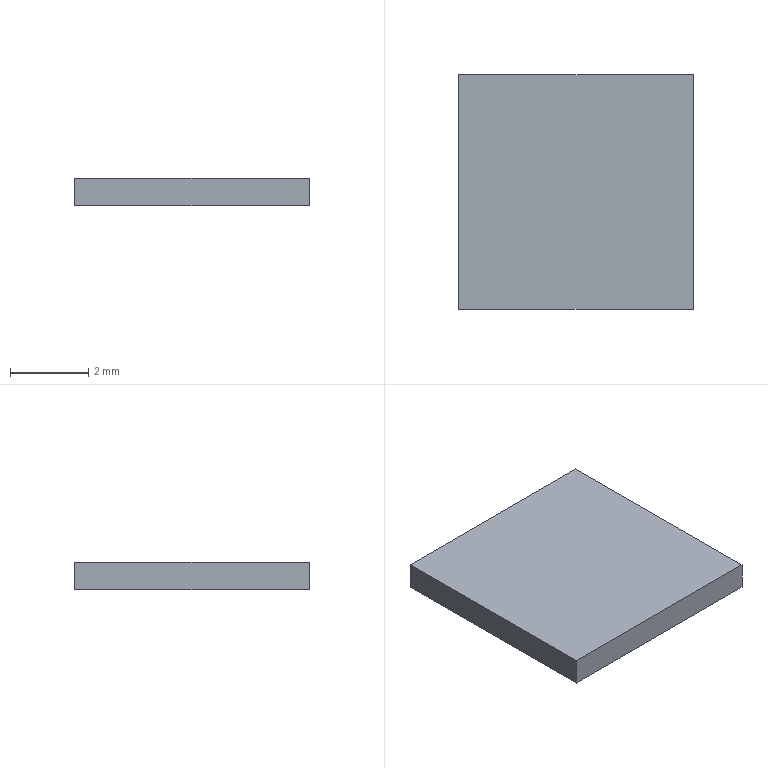Part | STEP file | RJ-USIO-V1_2-220411_378 | 1 solid | 6 faces | box 6 x 6 x 0.7 mm | volume 25.2 mm3 | plane 6
STEP:
#1=CARTESIAN_POINT('',(0.,0.,0.));
#2=DIRECTION('',(0.,0.,1.));
#3=DIRECTION('',(1.,0.,0.));
#4=AXIS2_PLACEMENT_3D('',#1,#2,#3);
#5=CARTESIAN_POINT('',(104.15,57.4,0.7));
#6=VERTEX_POINT('',#5);
#7=CARTESIAN_POINT('',(104.15,63.4,0.7));
#8=VERTEX_POINT('',#7);
#9=CARTESIAN_POINT('',(104.15,57.4,0.7));
#10=DIRECTION('',(-0.000000012,1.,0.));
#11=VECTOR('',#10,1.);
#12=LINE('',#9,#11);
#13=CARTESIAN_POINT('',(101.15,60.4,0.7));
#14=DIRECTION('',(0.,0.,1.));
#15=DIRECTION('',(-0.000000012,1.,0.));
#16=AXIS2_PLACEMENT_3D('',#13,#14,#15);
#17=PLANE('',#16);
#18=CARTESIAN_POINT('',(-3.,-3.));
#19=DIRECTION('',(1.,0.));
#20=VECTOR('',#19,1.);
#21=LINE('',#18,#20);
#22=(GEOMETRIC_REPRESENTATION_CONTEXT(2)PARAMETRIC_REPRESENTATION_CONTEXT()REPRESENTATION_CONTEXT('',''));
#23=DEFINITIONAL_REPRESENTATION('',(#21),#22);
#24=PCURVE('',#17,#23);
#25=CARTESIAN_POINT('',(104.15,60.4,0.35));
#26=DIRECTION('',(1.,0.000000012,0.));
#27=DIRECTION('',(0.,0.,1.));
#28=AXIS2_PLACEMENT_3D('',#25,#26,#27);
#29=PLANE('',#28);
#30=CARTESIAN_POINT('',(0.35,3.));
#31=DIRECTION('',(0.,-1.));
#32=VECTOR('',#31,1.);
#33=LINE('',#30,#32);
#34=(GEOMETRIC_REPRESENTATION_CONTEXT(2)PARAMETRIC_REPRESENTATION_CONTEXT()REPRESENTATION_CONTEXT('',''));
#35=DEFINITIONAL_REPRESENTATION('',(#33),#34);
#36=PCURVE('',#29,#35);
#37=SURFACE_CURVE('',#12,(#24,#36),.PCURVE_S1.);
#38=EDGE_CURVE('',#6,#8,#37,.T.);
#39=ORIENTED_EDGE('',*,*,#38,.F.);
#40=CARTESIAN_POINT('',(98.15,57.4,0.7));
#41=VERTEX_POINT('',#40);
#42=CARTESIAN_POINT('',(98.15,57.4,0.7));
#43=DIRECTION('',(1.,0.000000012,0.));
#44=VECTOR('',#43,1.);
#45=LINE('',#42,#44);
#46=CARTESIAN_POINT('',(-3.,3.));
#47=DIRECTION('',(0.,-1.));
#48=VECTOR('',#47,1.);
#49=LINE('',#46,#48);
#50=(GEOMETRIC_REPRESENTATION_CONTEXT(2)PARAMETRIC_REPRESENTATION_CONTEXT()REPRESENTATION_CONTEXT('',''));
#51=DEFINITIONAL_REPRESENTATION('',(#49),#50);
#52=PCURVE('',#17,#51);
#53=CARTESIAN_POINT('',(101.15,57.4,0.35));
#54=DIRECTION('',(0.000000012,-1.,0.));
#55=DIRECTION('',(0.,0.,-1.));
#56=AXIS2_PLACEMENT_3D('',#53,#54,#55);
#57=PLANE('',#56);
#58=CARTESIAN_POINT('',(-0.35,-3.));
#59=DIRECTION('',(0.,1.));
#60=VECTOR('',#59,1.);
#61=LINE('',#58,#60);
#62=(GEOMETRIC_REPRESENTATION_CONTEXT(2)PARAMETRIC_REPRESENTATION_CONTEXT()REPRESENTATION_CONTEXT('',''));
#63=DEFINITIONAL_REPRESENTATION('',(#61),#62);
#64=PCURVE('',#57,#63);
#65=SURFACE_CURVE('',#45,(#52,#64),.PCURVE_S1.);
#66=EDGE_CURVE('',#41,#6,#65,.T.);
#67=ORIENTED_EDGE('',*,*,#66,.F.);
#68=CARTESIAN_POINT('',(98.15,63.4,0.7));
#69=VERTEX_POINT('',#68);
#70=CARTESIAN_POINT('',(98.15,63.4,0.7));
#71=DIRECTION('',(0.000000012,-1.,0.));
#72=VECTOR('',#71,1.);
#73=LINE('',#70,#72);
#74=CARTESIAN_POINT('',(3.,3.));
#75=DIRECTION('',(-1.,0.));
#76=VECTOR('',#75,1.);
#77=LINE('',#74,#76);
#78=(GEOMETRIC_REPRESENTATION_CONTEXT(2)PARAMETRIC_REPRESENTATION_CONTEXT()REPRESENTATION_CONTEXT('',''));
#79=DEFINITIONAL_REPRESENTATION('',(#77),#78);
#80=PCURVE('',#17,#79);
#81=CARTESIAN_POINT('',(98.15,60.4,0.35));
#82=DIRECTION('',(1.,0.000000012,0.));
#83=DIRECTION('',(0.,0.,-1.));
#84=AXIS2_PLACEMENT_3D('',#81,#82,#83);
#85=PLANE('',#84);
#86=CARTESIAN_POINT('',(-0.35,3.));
#87=DIRECTION('',(0.,-1.));
#88=VECTOR('',#87,1.);
#89=LINE('',#86,#88);
#90=(GEOMETRIC_REPRESENTATION_CONTEXT(2)PARAMETRIC_REPRESENTATION_CONTEXT()REPRESENTATION_CONTEXT('',''));
#91=DEFINITIONAL_REPRESENTATION('',(#89),#90);
#92=PCURVE('',#85,#91);
#93=SURFACE_CURVE('',#73,(#80,#92),.PCURVE_S1.);
#94=EDGE_CURVE('',#69,#41,#93,.T.);
#95=ORIENTED_EDGE('',*,*,#94,.F.);
#96=CARTESIAN_POINT('',(104.15,63.4,0.7));
#97=DIRECTION('',(-1.,-0.000000012,0.));
#98=VECTOR('',#97,1.);
#99=LINE('',#96,#98);
#100=CARTESIAN_POINT('',(3.,-3.));
#101=DIRECTION('',(0.,1.));
#102=VECTOR('',#101,1.);
#103=LINE('',#100,#102);
#104=(GEOMETRIC_REPRESENTATION_CONTEXT(2)PARAMETRIC_REPRESENTATION_CONTEXT()REPRESENTATION_CONTEXT('',''));
#105=DEFINITIONAL_REPRESENTATION('',(#103),#104);
#106=PCURVE('',#17,#105);
#107=CARTESIAN_POINT('',(101.15,63.4,0.35));
#108=DIRECTION('',(0.000000012,-1.,0.));
#109=DIRECTION('',(0.,0.,1.));
#110=AXIS2_PLACEMENT_3D('',#107,#108,#109);
#111=PLANE('',#110);
#112=CARTESIAN_POINT('',(0.35,-3.));
#113=DIRECTION('',(0.,1.));
#114=VECTOR('',#113,1.);
#115=LINE('',#112,#114);
#116=(GEOMETRIC_REPRESENTATION_CONTEXT(2)PARAMETRIC_REPRESENTATION_CONTEXT()REPRESENTATION_CONTEXT('',''));
#117=DEFINITIONAL_REPRESENTATION('',(#115),#116);
#118=PCURVE('',#111,#117);
#119=SURFACE_CURVE('',#99,(#106,#118),.PCURVE_S1.);
#120=EDGE_CURVE('',#8,#69,#119,.T.);
#121=ORIENTED_EDGE('',*,*,#120,.F.);
#122=EDGE_LOOP('',(#39,#67,#95,#121));
#123=FACE_BOUND('',#122,.F.);
#124=ADVANCED_FACE('',(#123),#17,.T.);
#125=CARTESIAN_POINT('',(104.15,63.4,0.));
#126=VERTEX_POINT('',#125);
#127=CARTESIAN_POINT('',(104.15,63.4,0.7));
#128=DIRECTION('',(0.,0.,-1.));
#129=VECTOR('',#128,1.);
#130=LINE('',#127,#129);
#131=CARTESIAN_POINT('',(0.35,-3.));
#132=DIRECTION('',(-1.,0.));
#133=VECTOR('',#132,1.);
#134=LINE('',#131,#133);
#135=(GEOMETRIC_REPRESENTATION_CONTEXT(2)PARAMETRIC_REPRESENTATION_CONTEXT()REPRESENTATION_CONTEXT('',''));
#136=DEFINITIONAL_REPRESENTATION('',(#134),#135);
#137=PCURVE('',#29,#136);
#138=CARTESIAN_POINT('',(0.35,-3.));
#139=DIRECTION('',(-1.,0.));
#140=VECTOR('',#139,1.);
#141=LINE('',#138,#140);
#142=(GEOMETRIC_REPRESENTATION_CONTEXT(2)PARAMETRIC_REPRESENTATION_CONTEXT()REPRESENTATION_CONTEXT('',''));
#143=DEFINITIONAL_REPRESENTATION('',(#141),#142);
#144=PCURVE('',#111,#143);
#145=SURFACE_CURVE('',#130,(#137,#144),.PCURVE_S1.);
#146=EDGE_CURVE('',#8,#126,#145,.T.);
#147=ORIENTED_EDGE('',*,*,#146,.T.);
#148=CARTESIAN_POINT('',(104.15,57.4,0.));
#149=VERTEX_POINT('',#148);
#150=CARTESIAN_POINT('',(104.15,63.4,0.));
#151=DIRECTION('',(0.000000012,-1.,0.));
#152=VECTOR('',#151,1.);
#153=LINE('',#150,#152);
#154=CARTESIAN_POINT('',(-0.35,-3.));
#155=DIRECTION('',(0.,1.));
#156=VECTOR('',#155,1.);
#157=LINE('',#154,#156);
#158=(GEOMETRIC_REPRESENTATION_CONTEXT(2)PARAMETRIC_REPRESENTATION_CONTEXT()REPRESENTATION_CONTEXT('',''));
#159=DEFINITIONAL_REPRESENTATION('',(#157),#158);
#160=PCURVE('',#29,#159);
#161=CARTESIAN_POINT('',(101.15,60.4,0.));
#162=DIRECTION('',(0.,0.,1.));
#163=DIRECTION('',(-0.000000012,1.,0.));
#164=AXIS2_PLACEMENT_3D('',#161,#162,#163);
#165=PLANE('',#164);
#166=CARTESIAN_POINT('',(3.,-3.));
#167=DIRECTION('',(-1.,0.));
#168=VECTOR('',#167,1.);
#169=LINE('',#166,#168);
#170=(GEOMETRIC_REPRESENTATION_CONTEXT(2)PARAMETRIC_REPRESENTATION_CONTEXT()REPRESENTATION_CONTEXT('',''));
#171=DEFINITIONAL_REPRESENTATION('',(#169),#170);
#172=PCURVE('',#165,#171);
#173=SURFACE_CURVE('',#153,(#160,#172),.PCURVE_S1.);
#174=EDGE_CURVE('',#126,#149,#173,.T.);
#175=ORIENTED_EDGE('',*,*,#174,.T.);
#176=CARTESIAN_POINT('',(104.15,57.4,0.));
#177=DIRECTION('',(0.,0.,1.));
#178=VECTOR('',#177,1.);
#179=LINE('',#176,#178);
#180=CARTESIAN_POINT('',(-0.35,3.));
#181=DIRECTION('',(1.,0.));
#182=VECTOR('',#181,1.);
#183=LINE('',#180,#182);
#184=(GEOMETRIC_REPRESENTATION_CONTEXT(2)PARAMETRIC_REPRESENTATION_CONTEXT()REPRESENTATION_CONTEXT('',''));
#185=DEFINITIONAL_REPRESENTATION('',(#183),#184);
#186=PCURVE('',#29,#185);
#187=CARTESIAN_POINT('',(0.35,3.));
#188=DIRECTION('',(-1.,0.));
#189=VECTOR('',#188,1.);
#190=LINE('',#187,#189);
#191=(GEOMETRIC_REPRESENTATION_CONTEXT(2)PARAMETRIC_REPRESENTATION_CONTEXT()REPRESENTATION_CONTEXT('',''));
#192=DEFINITIONAL_REPRESENTATION('',(#190),#191);
#193=PCURVE('',#57,#192);
#194=SURFACE_CURVE('',#179,(#186,#193),.PCURVE_S1.);
#195=EDGE_CURVE('',#149,#6,#194,.T.);
#196=ORIENTED_EDGE('',*,*,#195,.T.);
#197=ORIENTED_EDGE('',*,*,#38,.T.);
#198=EDGE_LOOP('',(#147,#175,#196,#197));
#199=FACE_BOUND('',#198,.F.);
#200=ADVANCED_FACE('',(#199),#29,.T.);
#201=CARTESIAN_POINT('',(98.15,63.4,0.));
#202=VERTEX_POINT('',#201);
#203=CARTESIAN_POINT('',(98.15,63.4,0.));
#204=DIRECTION('',(0.,0.,1.));
#205=VECTOR('',#204,1.);
#206=LINE('',#203,#205);
#207=CARTESIAN_POINT('',(-0.35,3.));
#208=DIRECTION('',(1.,0.));
#209=VECTOR('',#208,1.);
#210=LINE('',#207,#209);
#211=(GEOMETRIC_REPRESENTATION_CONTEXT(2)PARAMETRIC_REPRESENTATION_CONTEXT()REPRESENTATION_CONTEXT('',''));
#212=DEFINITIONAL_REPRESENTATION('',(#210),#211);
#213=PCURVE('',#111,#212);
#214=CARTESIAN_POINT('',(0.35,3.));
#215=DIRECTION('',(-1.,0.));
#216=VECTOR('',#215,1.);
#217=LINE('',#214,#216);
#218=(GEOMETRIC_REPRESENTATION_CONTEXT(2)PARAMETRIC_REPRESENTATION_CONTEXT()REPRESENTATION_CONTEXT('',''));
#219=DEFINITIONAL_REPRESENTATION('',(#217),#218);
#220=PCURVE('',#85,#219);
#221=SURFACE_CURVE('',#206,(#213,#220),.PCURVE_S1.);
#222=EDGE_CURVE('',#202,#69,#221,.T.);
#223=ORIENTED_EDGE('',*,*,#222,.F.);
#224=CARTESIAN_POINT('',(98.15,63.4,0.));
#225=DIRECTION('',(1.,0.000000012,0.));
#226=VECTOR('',#225,1.);
#227=LINE('',#224,#226);
#228=CARTESIAN_POINT('',(-0.35,3.));
#229=DIRECTION('',(0.,-1.));
#230=VECTOR('',#229,1.);
#231=LINE('',#228,#230);
#232=(GEOMETRIC_REPRESENTATION_CONTEXT(2)PARAMETRIC_REPRESENTATION_CONTEXT()REPRESENTATION_CONTEXT('',''));
#233=DEFINITIONAL_REPRESENTATION('',(#231),#232);
#234=PCURVE('',#111,#233);
#235=CARTESIAN_POINT('',(3.,3.));
#236=DIRECTION('',(0.,-1.));
#237=VECTOR('',#236,1.);
#238=LINE('',#235,#237);
#239=(GEOMETRIC_REPRESENTATION_CONTEXT(2)PARAMETRIC_REPRESENTATION_CONTEXT()REPRESENTATION_CONTEXT('',''));
#240=DEFINITIONAL_REPRESENTATION('',(#238),#239);
#241=PCURVE('',#165,#240);
#242=SURFACE_CURVE('',#227,(#234,#241),.PCURVE_S1.);
#243=EDGE_CURVE('',#202,#126,#242,.T.);
#244=ORIENTED_EDGE('',*,*,#243,.T.);
#245=ORIENTED_EDGE('',*,*,#146,.F.);
#246=ORIENTED_EDGE('',*,*,#120,.T.);
#247=EDGE_LOOP('',(#223,#244,#245,#246));
#248=FACE_BOUND('',#247,.F.);
#249=ADVANCED_FACE('',(#248),#111,.F.);
#250=CARTESIAN_POINT('',(98.15,57.4,0.));
#251=VERTEX_POINT('',#250);
#252=CARTESIAN_POINT('',(98.15,57.4,0.));
#253=DIRECTION('',(0.,0.,1.));
#254=VECTOR('',#253,1.);
#255=LINE('',#252,#254);
#256=CARTESIAN_POINT('',(0.35,-3.));
#257=DIRECTION('',(-1.,0.));
#258=VECTOR('',#257,1.);
#259=LINE('',#256,#258);
#260=(GEOMETRIC_REPRESENTATION_CONTEXT(2)PARAMETRIC_REPRESENTATION_CONTEXT()REPRESENTATION_CONTEXT('',''));
#261=DEFINITIONAL_REPRESENTATION('',(#259),#260);
#262=PCURVE('',#85,#261);
#263=CARTESIAN_POINT('',(0.35,-3.));
#264=DIRECTION('',(-1.,0.));
#265=VECTOR('',#264,1.);
#266=LINE('',#263,#265);
#267=(GEOMETRIC_REPRESENTATION_CONTEXT(2)PARAMETRIC_REPRESENTATION_CONTEXT()REPRESENTATION_CONTEXT('',''));
#268=DEFINITIONAL_REPRESENTATION('',(#266),#267);
#269=PCURVE('',#57,#268);
#270=SURFACE_CURVE('',#255,(#262,#269),.PCURVE_S1.);
#271=EDGE_CURVE('',#251,#41,#270,.T.);
#272=ORIENTED_EDGE('',*,*,#271,.F.);
#273=CARTESIAN_POINT('',(98.15,57.4,0.));
#274=DIRECTION('',(-0.000000012,1.,0.));
#275=VECTOR('',#274,1.);
#276=LINE('',#273,#275);
#277=CARTESIAN_POINT('',(0.35,-3.));
#278=DIRECTION('',(0.,1.));
#279=VECTOR('',#278,1.);
#280=LINE('',#277,#279);
#281=(GEOMETRIC_REPRESENTATION_CONTEXT(2)PARAMETRIC_REPRESENTATION_CONTEXT()REPRESENTATION_CONTEXT('',''));
#282=DEFINITIONAL_REPRESENTATION('',(#280),#281);
#283=PCURVE('',#85,#282);
#284=CARTESIAN_POINT('',(-3.,3.));
#285=DIRECTION('',(1.,0.));
#286=VECTOR('',#285,1.);
#287=LINE('',#284,#286);
#288=(GEOMETRIC_REPRESENTATION_CONTEXT(2)PARAMETRIC_REPRESENTATION_CONTEXT()REPRESENTATION_CONTEXT('',''));
#289=DEFINITIONAL_REPRESENTATION('',(#287),#288);
#290=PCURVE('',#165,#289);
#291=SURFACE_CURVE('',#276,(#283,#290),.PCURVE_S1.);
#292=EDGE_CURVE('',#251,#202,#291,.T.);
#293=ORIENTED_EDGE('',*,*,#292,.T.);
#294=ORIENTED_EDGE('',*,*,#222,.T.);
#295=ORIENTED_EDGE('',*,*,#94,.T.);
#296=EDGE_LOOP('',(#272,#293,#294,#295));
#297=FACE_BOUND('',#296,.F.);
#298=ADVANCED_FACE('',(#297),#85,.F.);
#299=ORIENTED_EDGE('',*,*,#195,.F.);
#300=CARTESIAN_POINT('',(104.15,57.4,0.));
#301=DIRECTION('',(-1.,-0.000000012,0.));
#302=VECTOR('',#301,1.);
#303=LINE('',#300,#302);
#304=CARTESIAN_POINT('',(0.35,3.));
#305=DIRECTION('',(0.,-1.));
#306=VECTOR('',#305,1.);
#307=LINE('',#304,#306);
#308=(GEOMETRIC_REPRESENTATION_CONTEXT(2)PARAMETRIC_REPRESENTATION_CONTEXT()REPRESENTATION_CONTEXT('',''));
#309=DEFINITIONAL_REPRESENTATION('',(#307),#308);
#310=PCURVE('',#57,#309);
#311=CARTESIAN_POINT('',(-3.,-3.));
#312=DIRECTION('',(0.,1.));
#313=VECTOR('',#312,1.);
#314=LINE('',#311,#313);
#315=(GEOMETRIC_REPRESENTATION_CONTEXT(2)PARAMETRIC_REPRESENTATION_CONTEXT()REPRESENTATION_CONTEXT('',''));
#316=DEFINITIONAL_REPRESENTATION('',(#314),#315);
#317=PCURVE('',#165,#316);
#318=SURFACE_CURVE('',#303,(#310,#317),.PCURVE_S1.);
#319=EDGE_CURVE('',#149,#251,#318,.T.);
#320=ORIENTED_EDGE('',*,*,#319,.T.);
#321=ORIENTED_EDGE('',*,*,#271,.T.);
#322=ORIENTED_EDGE('',*,*,#66,.T.);
#323=EDGE_LOOP('',(#299,#320,#321,#322));
#324=FACE_BOUND('',#323,.F.);
#325=ADVANCED_FACE('',(#324),#57,.T.);
#326=ORIENTED_EDGE('',*,*,#174,.F.);
#327=ORIENTED_EDGE('',*,*,#243,.F.);
#328=ORIENTED_EDGE('',*,*,#292,.F.);
#329=ORIENTED_EDGE('',*,*,#319,.F.);
#330=EDGE_LOOP('',(#326,#327,#328,#329));
#331=FACE_BOUND('',#330,.F.);
#332=ADVANCED_FACE('',(#331),#165,.F.);
#333=CLOSED_SHELL('',(#124,#200,#249,#298,#325,#332));
#334=MANIFOLD_SOLID_BREP('',#333);
#335=(LENGTH_UNIT()NAMED_UNIT(*)SI_UNIT(.MILLI.,.METRE.));
#336=UNCERTAINTY_MEASURE_WITH_UNIT(LENGTH_MEASURE(0.0000001),#335,'','');
#337=(NAMED_UNIT(*)PLANE_ANGLE_UNIT()SI_UNIT($,.RADIAN.));
#338=(NAMED_UNIT(*)SI_UNIT($,.STERADIAN.)SOLID_ANGLE_UNIT());
#339=(GEOMETRIC_REPRESENTATION_CONTEXT(3)GLOBAL_UNCERTAINTY_ASSIGNED_CONTEXT((#336))GLOBAL_UNIT_ASSIGNED_CONTEXT((#335,#337,#338))REPRESENTATION_CONTEXT('',''));
#340=ADVANCED_BREP_SHAPE_REPRESENTATION('',(#4,#334),#339);